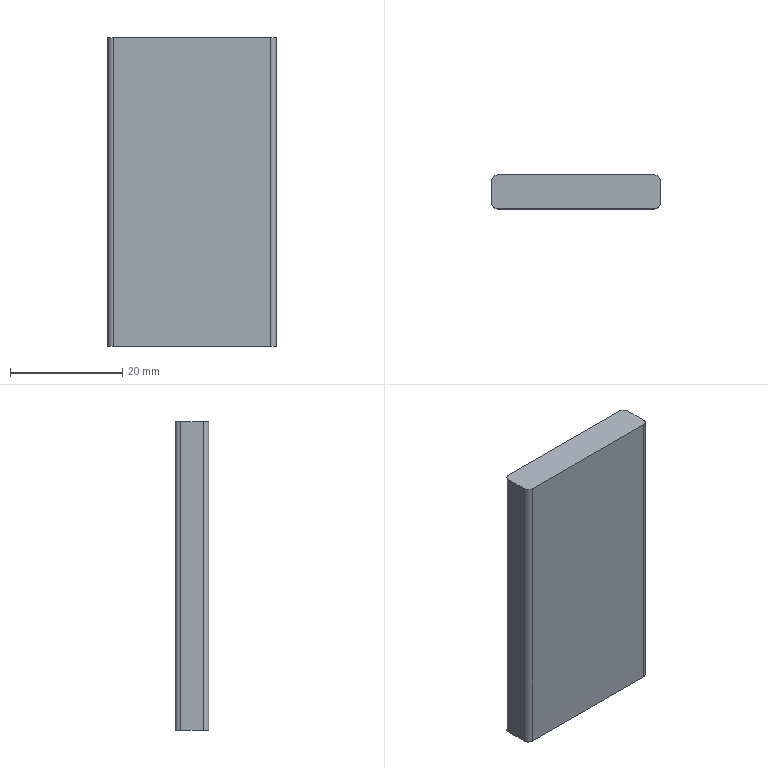Part | STEP file | 1 solid | 10 faces | box 29.97 x 5.97 x 55 mm | volume 9793 mm3 | plane 6 | cylinder 4 | commonest cylinder face diameters 2 x4
STEP:
#1=CARTESIAN_POINT('',(0.,0.,0.));
#2=DIRECTION('',(0.,0.,1.));
#3=DIRECTION('',(1.,0.,0.));
#4=AXIS2_PLACEMENT_3D('',#1,#2,#3);
#5=CARTESIAN_POINT('',(1284.232,493.53,43.619));
#6=VERTEX_POINT('',#5);
#7=CARTESIAN_POINT('',(1256.262,493.53,43.619));
#8=VERTEX_POINT('',#7);
#9=CARTESIAN_POINT('',(1285.247,493.53,43.619));
#10=DIRECTION('',(-1.,0.,0.));
#11=VECTOR('',#10,1.);
#12=LINE('',#9,#11);
#13=CARTESIAN_POINT('',(20687.4,-3520.314,43.619));
#14=DIRECTION('',(0.,0.,1.));
#15=DIRECTION('',(1.,0.,0.));
#16=AXIS2_PLACEMENT_3D('',#13,#14,#15);
#17=PLANE('',#16);
#18=CARTESIAN_POINT('',(-19402.153,4013.844));
#19=DIRECTION('',(-1.,0.));
#20=VECTOR('',#19,1.);
#21=LINE('',#18,#20);
#22=(GEOMETRIC_REPRESENTATION_CONTEXT(2)PARAMETRIC_REPRESENTATION_CONTEXT()REPRESENTATION_CONTEXT('',''));
#23=DEFINITIONAL_REPRESENTATION('',(#21),#22);
#24=PCURVE('',#17,#23);
#25=CARTESIAN_POINT('',(1285.247,493.53,426.319));
#26=DIRECTION('',(0.,-1.,0.));
#27=DIRECTION('',(0.,0.,1.));
#28=AXIS2_PLACEMENT_3D('',#25,#26,#27);
#29=PLANE('',#28);
#30=CARTESIAN_POINT('',(-382.7,0.));
#31=DIRECTION('',(0.,1.));
#32=VECTOR('',#31,1.);
#33=LINE('',#30,#32);
#34=(GEOMETRIC_REPRESENTATION_CONTEXT(2)PARAMETRIC_REPRESENTATION_CONTEXT()REPRESENTATION_CONTEXT('',''));
#35=DEFINITIONAL_REPRESENTATION('',(#33),#34);
#36=PCURVE('',#29,#35);
#37=SURFACE_CURVE('',#12,(#24,#36),.PCURVE_S1.);
#38=EDGE_CURVE('',#6,#8,#37,.T.);
#39=ORIENTED_EDGE('',*,*,#38,.T.);
#40=CARTESIAN_POINT('',(1255.262,492.53,43.619));
#41=VERTEX_POINT('',#40);
#42=CARTESIAN_POINT('',(1256.262,492.53,43.619));
#43=DIRECTION('',(0.,0.,1.));
#44=DIRECTION('',(-1.,0.,0.));
#45=AXIS2_PLACEMENT_3D('',#42,#43,#44);
#46=CIRCLE('',#45,1.);
#47=CARTESIAN_POINT('',(-19431.138,4012.844));
#48=DIRECTION('',(-1.,0.));
#49=AXIS2_PLACEMENT_2D('',#47,#48);
#50=CIRCLE('',#49,1.);
#51=(GEOMETRIC_REPRESENTATION_CONTEXT(2)PARAMETRIC_REPRESENTATION_CONTEXT()REPRESENTATION_CONTEXT('',''));
#52=DEFINITIONAL_REPRESENTATION('',(#50),#51);
#53=PCURVE('',#17,#52);
#54=CARTESIAN_POINT('',(1256.262,492.53,426.319));
#55=DIRECTION('',(0.,0.,-1.));
#56=DIRECTION('',(-1.,0.,0.));
#57=AXIS2_PLACEMENT_3D('',#54,#55,#56);
#58=CYLINDRICAL_SURFACE('',#57,1.);
#59=CARTESIAN_POINT('',(6.283,382.7));
#60=DIRECTION('',(-1.,0.));
#61=VECTOR('',#60,1.);
#62=LINE('',#59,#61);
#63=(GEOMETRIC_REPRESENTATION_CONTEXT(2)PARAMETRIC_REPRESENTATION_CONTEXT()REPRESENTATION_CONTEXT('',''));
#64=DEFINITIONAL_REPRESENTATION('',(#62),#63);
#65=PCURVE('',#58,#64);
#66=SURFACE_CURVE('',#46,(#53,#65),.PCURVE_S1.);
#67=EDGE_CURVE('',#8,#41,#66,.T.);
#68=ORIENTED_EDGE('',*,*,#67,.T.);
#69=CARTESIAN_POINT('',(1255.262,488.56,43.619));
#70=VERTEX_POINT('',#69);
#71=CARTESIAN_POINT('',(1255.262,493.545,43.619));
#72=DIRECTION('',(0.,-1.,0.));
#73=VECTOR('',#72,1.);
#74=LINE('',#71,#73);
#75=CARTESIAN_POINT('',(-19432.138,4013.859));
#76=DIRECTION('',(0.,-1.));
#77=VECTOR('',#76,1.);
#78=LINE('',#75,#77);
#79=(GEOMETRIC_REPRESENTATION_CONTEXT(2)PARAMETRIC_REPRESENTATION_CONTEXT()REPRESENTATION_CONTEXT('',''));
#80=DEFINITIONAL_REPRESENTATION('',(#78),#79);
#81=PCURVE('',#17,#80);
#82=CARTESIAN_POINT('',(1255.262,493.545,426.319));
#83=DIRECTION('',(1.,0.,0.));
#84=DIRECTION('',(0.,0.,-1.));
#85=AXIS2_PLACEMENT_3D('',#82,#83,#84);
#86=PLANE('',#85);
#87=CARTESIAN_POINT('',(382.7,0.));
#88=DIRECTION('',(0.,-1.));
#89=VECTOR('',#88,1.);
#90=LINE('',#87,#89);
#91=(GEOMETRIC_REPRESENTATION_CONTEXT(2)PARAMETRIC_REPRESENTATION_CONTEXT()REPRESENTATION_CONTEXT('',''));
#92=DEFINITIONAL_REPRESENTATION('',(#90),#91);
#93=PCURVE('',#86,#92);
#94=SURFACE_CURVE('',#74,(#81,#93),.PCURVE_S1.);
#95=EDGE_CURVE('',#41,#70,#94,.T.);
#96=ORIENTED_EDGE('',*,*,#95,.T.);
#97=CARTESIAN_POINT('',(1256.262,487.56,43.619));
#98=VERTEX_POINT('',#97);
#99=CARTESIAN_POINT('',(1256.262,488.56,43.619));
#100=DIRECTION('',(0.,0.,1.));
#101=DIRECTION('',(-1.,0.,0.));
#102=AXIS2_PLACEMENT_3D('',#99,#100,#101);
#103=CIRCLE('',#102,1.);
#104=CARTESIAN_POINT('',(-19431.138,4008.874));
#105=DIRECTION('',(-1.,0.));
#106=AXIS2_PLACEMENT_2D('',#104,#105);
#107=CIRCLE('',#106,1.);
#108=(GEOMETRIC_REPRESENTATION_CONTEXT(2)PARAMETRIC_REPRESENTATION_CONTEXT()REPRESENTATION_CONTEXT('',''));
#109=DEFINITIONAL_REPRESENTATION('',(#107),#108);
#110=PCURVE('',#17,#109);
#111=CARTESIAN_POINT('',(1256.262,488.56,426.319));
#112=DIRECTION('',(0.,0.,-1.));
#113=DIRECTION('',(-1.,0.,0.));
#114=AXIS2_PLACEMENT_3D('',#111,#112,#113);
#115=CYLINDRICAL_SURFACE('',#114,1.);
#116=CARTESIAN_POINT('',(6.283,382.7));
#117=DIRECTION('',(-1.,0.));
#118=VECTOR('',#117,1.);
#119=LINE('',#116,#118);
#120=(GEOMETRIC_REPRESENTATION_CONTEXT(2)PARAMETRIC_REPRESENTATION_CONTEXT()REPRESENTATION_CONTEXT('',''));
#121=DEFINITIONAL_REPRESENTATION('',(#119),#120);
#122=PCURVE('',#115,#121);
#123=SURFACE_CURVE('',#103,(#110,#122),.PCURVE_S1.);
#124=EDGE_CURVE('',#70,#98,#123,.T.);
#125=ORIENTED_EDGE('',*,*,#124,.T.);
#126=CARTESIAN_POINT('',(1284.232,487.56,43.619));
#127=VERTEX_POINT('',#126);
#128=CARTESIAN_POINT('',(1255.247,487.56,43.619));
#129=DIRECTION('',(1.,0.,0.));
#130=VECTOR('',#129,1.);
#131=LINE('',#128,#130);
#132=CARTESIAN_POINT('',(-19432.153,4007.874));
#133=DIRECTION('',(1.,0.));
#134=VECTOR('',#133,1.);
#135=LINE('',#132,#134);
#136=(GEOMETRIC_REPRESENTATION_CONTEXT(2)PARAMETRIC_REPRESENTATION_CONTEXT()REPRESENTATION_CONTEXT('',''));
#137=DEFINITIONAL_REPRESENTATION('',(#135),#136);
#138=PCURVE('',#17,#137);
#139=CARTESIAN_POINT('',(1255.247,487.56,426.319));
#140=DIRECTION('',(0.,1.,0.));
#141=DIRECTION('',(0.,0.,-1.));
#142=AXIS2_PLACEMENT_3D('',#139,#140,#141);
#143=PLANE('',#142);
#144=CARTESIAN_POINT('',(382.7,0.));
#145=DIRECTION('',(0.,-1.));
#146=VECTOR('',#145,1.);
#147=LINE('',#144,#146);
#148=(GEOMETRIC_REPRESENTATION_CONTEXT(2)PARAMETRIC_REPRESENTATION_CONTEXT()REPRESENTATION_CONTEXT('',''));
#149=DEFINITIONAL_REPRESENTATION('',(#147),#148);
#150=PCURVE('',#143,#149);
#151=SURFACE_CURVE('',#131,(#138,#150),.PCURVE_S1.);
#152=EDGE_CURVE('',#98,#127,#151,.T.);
#153=ORIENTED_EDGE('',*,*,#152,.T.);
#154=CARTESIAN_POINT('',(1285.232,488.56,43.619));
#155=VERTEX_POINT('',#154);
#156=CARTESIAN_POINT('',(1284.232,488.56,43.619));
#157=DIRECTION('',(0.,0.,1.));
#158=DIRECTION('',(-1.,0.,0.));
#159=AXIS2_PLACEMENT_3D('',#156,#157,#158);
#160=CIRCLE('',#159,1.);
#161=CARTESIAN_POINT('',(-19403.168,4008.874));
#162=DIRECTION('',(-1.,0.));
#163=AXIS2_PLACEMENT_2D('',#161,#162);
#164=CIRCLE('',#163,1.);
#165=(GEOMETRIC_REPRESENTATION_CONTEXT(2)PARAMETRIC_REPRESENTATION_CONTEXT()REPRESENTATION_CONTEXT('',''));
#166=DEFINITIONAL_REPRESENTATION('',(#164),#165);
#167=PCURVE('',#17,#166);
#168=CARTESIAN_POINT('',(1284.232,488.56,426.319));
#169=DIRECTION('',(0.,0.,-1.));
#170=DIRECTION('',(-1.,0.,0.));
#171=AXIS2_PLACEMENT_3D('',#168,#169,#170);
#172=CYLINDRICAL_SURFACE('',#171,1.);
#173=CARTESIAN_POINT('',(6.283,382.7));
#174=DIRECTION('',(-1.,0.));
#175=VECTOR('',#174,1.);
#176=LINE('',#173,#175);
#177=(GEOMETRIC_REPRESENTATION_CONTEXT(2)PARAMETRIC_REPRESENTATION_CONTEXT()REPRESENTATION_CONTEXT('',''));
#178=DEFINITIONAL_REPRESENTATION('',(#176),#177);
#179=PCURVE('',#172,#178);
#180=SURFACE_CURVE('',#160,(#167,#179),.PCURVE_S1.);
#181=EDGE_CURVE('',#127,#155,#180,.T.);
#182=ORIENTED_EDGE('',*,*,#181,.T.);
#183=CARTESIAN_POINT('',(1285.232,492.53,43.619));
#184=VERTEX_POINT('',#183);
#185=CARTESIAN_POINT('',(1285.232,487.545,43.619));
#186=DIRECTION('',(0.,1.,0.));
#187=VECTOR('',#186,1.);
#188=LINE('',#185,#187);
#189=CARTESIAN_POINT('',(-19402.168,4007.859));
#190=DIRECTION('',(0.,1.));
#191=VECTOR('',#190,1.);
#192=LINE('',#189,#191);
#193=(GEOMETRIC_REPRESENTATION_CONTEXT(2)PARAMETRIC_REPRESENTATION_CONTEXT()REPRESENTATION_CONTEXT('',''));
#194=DEFINITIONAL_REPRESENTATION('',(#192),#193);
#195=PCURVE('',#17,#194);
#196=CARTESIAN_POINT('',(1285.232,487.545,426.319));
#197=DIRECTION('',(-1.,0.,0.));
#198=DIRECTION('',(0.,0.,1.));
#199=AXIS2_PLACEMENT_3D('',#196,#197,#198);
#200=PLANE('',#199);
#201=CARTESIAN_POINT('',(-382.7,0.));
#202=DIRECTION('',(0.,1.));
#203=VECTOR('',#202,1.);
#204=LINE('',#201,#203);
#205=(GEOMETRIC_REPRESENTATION_CONTEXT(2)PARAMETRIC_REPRESENTATION_CONTEXT()REPRESENTATION_CONTEXT('',''));
#206=DEFINITIONAL_REPRESENTATION('',(#204),#205);
#207=PCURVE('',#200,#206);
#208=SURFACE_CURVE('',#188,(#195,#207),.PCURVE_S1.);
#209=EDGE_CURVE('',#155,#184,#208,.T.);
#210=ORIENTED_EDGE('',*,*,#209,.T.);
#211=CARTESIAN_POINT('',(1284.232,492.53,43.619));
#212=DIRECTION('',(0.,0.,1.));
#213=DIRECTION('',(-1.,0.,0.));
#214=AXIS2_PLACEMENT_3D('',#211,#212,#213);
#215=CIRCLE('',#214,1.);
#216=CARTESIAN_POINT('',(-19403.168,4012.844));
#217=DIRECTION('',(-1.,0.));
#218=AXIS2_PLACEMENT_2D('',#216,#217);
#219=CIRCLE('',#218,1.);
#220=(GEOMETRIC_REPRESENTATION_CONTEXT(2)PARAMETRIC_REPRESENTATION_CONTEXT()REPRESENTATION_CONTEXT('',''));
#221=DEFINITIONAL_REPRESENTATION('',(#219),#220);
#222=PCURVE('',#17,#221);
#223=CARTESIAN_POINT('',(1284.232,492.53,426.319));
#224=DIRECTION('',(0.,0.,-1.));
#225=DIRECTION('',(-1.,0.,0.));
#226=AXIS2_PLACEMENT_3D('',#223,#224,#225);
#227=CYLINDRICAL_SURFACE('',#226,1.);
#228=CARTESIAN_POINT('',(6.283,382.7));
#229=DIRECTION('',(-1.,0.));
#230=VECTOR('',#229,1.);
#231=LINE('',#228,#230);
#232=(GEOMETRIC_REPRESENTATION_CONTEXT(2)PARAMETRIC_REPRESENTATION_CONTEXT()REPRESENTATION_CONTEXT('',''));
#233=DEFINITIONAL_REPRESENTATION('',(#231),#232);
#234=PCURVE('',#227,#233);
#235=SURFACE_CURVE('',#215,(#222,#234),.PCURVE_S1.);
#236=EDGE_CURVE('',#184,#6,#235,.T.);
#237=ORIENTED_EDGE('',*,*,#236,.T.);
#238=EDGE_LOOP('',(#39,#68,#96,#125,#153,#182,#210,#237));
#239=FACE_BOUND('',#238,.T.);
#240=ADVANCED_FACE('',(#239),#17,.T.);
#241=CARTESIAN_POINT('',(1284.232,493.53,-11.381));
#242=VERTEX_POINT('',#241);
#243=CARTESIAN_POINT('',(1256.262,493.53,-11.381));
#244=VERTEX_POINT('',#243);
#245=CARTESIAN_POINT('',(1285.247,493.53,-11.381));
#246=DIRECTION('',(-1.,0.,0.));
#247=VECTOR('',#246,1.);
#248=LINE('',#245,#247);
#249=CARTESIAN_POINT('',(-437.7,0.));
#250=DIRECTION('',(0.,1.));
#251=VECTOR('',#250,1.);
#252=LINE('',#249,#251);
#253=(GEOMETRIC_REPRESENTATION_CONTEXT(2)PARAMETRIC_REPRESENTATION_CONTEXT()REPRESENTATION_CONTEXT('',''));
#254=DEFINITIONAL_REPRESENTATION('',(#252),#253);
#255=PCURVE('',#29,#254);
#256=CARTESIAN_POINT('',(18450.131,-3520.314,-11.381));
#257=DIRECTION('',(0.,0.,1.));
#258=DIRECTION('',(1.,0.,0.));
#259=AXIS2_PLACEMENT_3D('',#256,#257,#258);
#260=PLANE('',#259);
#261=CARTESIAN_POINT('',(-17164.884,4013.844));
#262=DIRECTION('',(-1.,0.));
#263=VECTOR('',#262,1.);
#264=LINE('',#261,#263);
#265=(GEOMETRIC_REPRESENTATION_CONTEXT(2)PARAMETRIC_REPRESENTATION_CONTEXT()REPRESENTATION_CONTEXT('',''));
#266=DEFINITIONAL_REPRESENTATION('',(#264),#265);
#267=PCURVE('',#260,#266);
#268=SURFACE_CURVE('',#248,(#255,#267),.PCURVE_S1.);
#269=EDGE_CURVE('',#242,#244,#268,.T.);
#270=ORIENTED_EDGE('',*,*,#269,.T.);
#271=CARTESIAN_POINT('',(1256.262,493.53,426.319));
#272=DIRECTION('',(0.,0.,1.));
#273=VECTOR('',#272,1.);
#274=LINE('',#271,#273);
#275=CARTESIAN_POINT('',(0.,28.985));
#276=DIRECTION('',(1.,0.));
#277=VECTOR('',#276,1.);
#278=LINE('',#275,#277);
#279=(GEOMETRIC_REPRESENTATION_CONTEXT(2)PARAMETRIC_REPRESENTATION_CONTEXT()REPRESENTATION_CONTEXT('',''));
#280=DEFINITIONAL_REPRESENTATION('',(#278),#279);
#281=PCURVE('',#29,#280);
#282=CARTESIAN_POINT('',(1.571,0.));
#283=DIRECTION('',(0.,-1.));
#284=VECTOR('',#283,1.);
#285=LINE('',#282,#284);
#286=(GEOMETRIC_REPRESENTATION_CONTEXT(2)PARAMETRIC_REPRESENTATION_CONTEXT()REPRESENTATION_CONTEXT('',''));
#287=DEFINITIONAL_REPRESENTATION('',(#285),#286);
#288=PCURVE('',#58,#287);
#289=SURFACE_CURVE('',#274,(#281,#288),.PCURVE_S1.);
#290=EDGE_CURVE('',#244,#8,#289,.T.);
#291=ORIENTED_EDGE('',*,*,#290,.T.);
#292=ORIENTED_EDGE('',*,*,#38,.F.);
#293=CARTESIAN_POINT('',(1284.232,493.53,426.319));
#294=DIRECTION('',(0.,0.,-1.));
#295=VECTOR('',#294,1.);
#296=LINE('',#293,#295);
#297=CARTESIAN_POINT('',(0.,1.015));
#298=DIRECTION('',(-1.,0.));
#299=VECTOR('',#298,1.);
#300=LINE('',#297,#299);
#301=(GEOMETRIC_REPRESENTATION_CONTEXT(2)PARAMETRIC_REPRESENTATION_CONTEXT()REPRESENTATION_CONTEXT('',''));
#302=DEFINITIONAL_REPRESENTATION('',(#300),#301);
#303=PCURVE('',#29,#302);
#304=CARTESIAN_POINT('',(1.571,0.));
#305=DIRECTION('',(0.,1.));
#306=VECTOR('',#305,1.);
#307=LINE('',#304,#306);
#308=(GEOMETRIC_REPRESENTATION_CONTEXT(2)PARAMETRIC_REPRESENTATION_CONTEXT()REPRESENTATION_CONTEXT('',''));
#309=DEFINITIONAL_REPRESENTATION('',(#307),#308);
#310=PCURVE('',#227,#309);
#311=SURFACE_CURVE('',#296,(#303,#310),.PCURVE_S1.);
#312=EDGE_CURVE('',#6,#242,#311,.T.);
#313=ORIENTED_EDGE('',*,*,#312,.T.);
#314=EDGE_LOOP('',(#270,#291,#292,#313));
#315=FACE_BOUND('',#314,.T.);
#316=ADVANCED_FACE('',(#315),#29,.F.);
#317=ORIENTED_EDGE('',*,*,#95,.F.);
#318=CARTESIAN_POINT('',(1255.262,492.53,-11.381));
#319=VERTEX_POINT('',#318);
#320=CARTESIAN_POINT('',(1255.262,492.53,426.319));
#321=DIRECTION('',(0.,0.,-1.));
#322=VECTOR('',#321,1.);
#323=LINE('',#320,#322);
#324=CARTESIAN_POINT('',(0.,-1.015));
#325=DIRECTION('',(1.,0.));
#326=VECTOR('',#325,1.);
#327=LINE('',#324,#326);
#328=(GEOMETRIC_REPRESENTATION_CONTEXT(2)PARAMETRIC_REPRESENTATION_CONTEXT()REPRESENTATION_CONTEXT('',''));
#329=DEFINITIONAL_REPRESENTATION('',(#327),#328);
#330=PCURVE('',#86,#329);
#331=CARTESIAN_POINT('',(0.,0.));
#332=DIRECTION('',(0.,1.));
#333=VECTOR('',#332,1.);
#334=LINE('',#331,#333);
#335=(GEOMETRIC_REPRESENTATION_CONTEXT(2)PARAMETRIC_REPRESENTATION_CONTEXT()REPRESENTATION_CONTEXT('',''));
#336=DEFINITIONAL_REPRESENTATION('',(#334),#335);
#337=PCURVE('',#58,#336);
#338=SURFACE_CURVE('',#323,(#330,#337),.PCURVE_S1.);
#339=EDGE_CURVE('',#41,#319,#338,.T.);
#340=ORIENTED_EDGE('',*,*,#339,.T.);
#341=CARTESIAN_POINT('',(1255.262,488.56,-11.381));
#342=VERTEX_POINT('',#341);
#343=CARTESIAN_POINT('',(1255.262,493.545,-11.381));
#344=DIRECTION('',(0.,-1.,0.));
#345=VECTOR('',#344,1.);
#346=LINE('',#343,#345);
#347=CARTESIAN_POINT('',(437.7,0.));
#348=DIRECTION('',(0.,-1.));
#349=VECTOR('',#348,1.);
#350=LINE('',#347,#349);
#351=(GEOMETRIC_REPRESENTATION_CONTEXT(2)PARAMETRIC_REPRESENTATION_CONTEXT()REPRESENTATION_CONTEXT('',''));
#352=DEFINITIONAL_REPRESENTATION('',(#350),#351);
#353=PCURVE('',#86,#352);
#354=CARTESIAN_POINT('',(-17194.869,4013.859));
#355=DIRECTION('',(0.,-1.));
#356=VECTOR('',#355,1.);
#357=LINE('',#354,#356);
#358=(GEOMETRIC_REPRESENTATION_CONTEXT(2)PARAMETRIC_REPRESENTATION_CONTEXT()REPRESENTATION_CONTEXT('',''));
#359=DEFINITIONAL_REPRESENTATION('',(#357),#358);
#360=PCURVE('',#260,#359);
#361=SURFACE_CURVE('',#346,(#353,#360),.PCURVE_S1.);
#362=EDGE_CURVE('',#319,#342,#361,.T.);
#363=ORIENTED_EDGE('',*,*,#362,.T.);
#364=CARTESIAN_POINT('',(1255.262,488.56,426.319));
#365=DIRECTION('',(0.,0.,1.));
#366=VECTOR('',#365,1.);
#367=LINE('',#364,#366);
#368=CARTESIAN_POINT('',(0.,-4.985));
#369=DIRECTION('',(-1.,0.));
#370=VECTOR('',#369,1.);
#371=LINE('',#368,#370);
#372=(GEOMETRIC_REPRESENTATION_CONTEXT(2)PARAMETRIC_REPRESENTATION_CONTEXT()REPRESENTATION_CONTEXT('',''));
#373=DEFINITIONAL_REPRESENTATION('',(#371),#372);
#374=PCURVE('',#86,#373);
#375=CARTESIAN_POINT('',(6.283,0.));
#376=DIRECTION('',(0.,-1.));
#377=VECTOR('',#376,1.);
#378=LINE('',#375,#377);
#379=(GEOMETRIC_REPRESENTATION_CONTEXT(2)PARAMETRIC_REPRESENTATION_CONTEXT()REPRESENTATION_CONTEXT('',''));
#380=DEFINITIONAL_REPRESENTATION('',(#378),#379);
#381=PCURVE('',#115,#380);
#382=SURFACE_CURVE('',#367,(#374,#381),.PCURVE_S1.);
#383=EDGE_CURVE('',#342,#70,#382,.T.);
#384=ORIENTED_EDGE('',*,*,#383,.T.);
#385=EDGE_LOOP('',(#317,#340,#363,#384));
#386=FACE_BOUND('',#385,.T.);
#387=ADVANCED_FACE('',(#386),#86,.F.);
#388=ORIENTED_EDGE('',*,*,#152,.F.);
#389=CARTESIAN_POINT('',(1256.262,487.56,-11.381));
#390=VERTEX_POINT('',#389);
#391=CARTESIAN_POINT('',(1256.262,487.56,426.319));
#392=DIRECTION('',(0.,0.,-1.));
#393=VECTOR('',#392,1.);
#394=LINE('',#391,#393);
#395=CARTESIAN_POINT('',(0.,-1.015));
#396=DIRECTION('',(1.,0.));
#397=VECTOR('',#396,1.);
#398=LINE('',#395,#397);
#399=(GEOMETRIC_REPRESENTATION_CONTEXT(2)PARAMETRIC_REPRESENTATION_CONTEXT()REPRESENTATION_CONTEXT('',''));
#400=DEFINITIONAL_REPRESENTATION('',(#398),#399);
#401=PCURVE('',#143,#400);
#402=CARTESIAN_POINT('',(4.712,0.));
#403=DIRECTION('',(0.,1.));
#404=VECTOR('',#403,1.);
#405=LINE('',#402,#404);
#406=(GEOMETRIC_REPRESENTATION_CONTEXT(2)PARAMETRIC_REPRESENTATION_CONTEXT()REPRESENTATION_CONTEXT('',''));
#407=DEFINITIONAL_REPRESENTATION('',(#405),#406);
#408=PCURVE('',#115,#407);
#409=SURFACE_CURVE('',#394,(#401,#408),.PCURVE_S1.);
#410=EDGE_CURVE('',#98,#390,#409,.T.);
#411=ORIENTED_EDGE('',*,*,#410,.T.);
#412=CARTESIAN_POINT('',(1284.232,487.56,-11.381));
#413=VERTEX_POINT('',#412);
#414=CARTESIAN_POINT('',(1255.247,487.56,-11.381));
#415=DIRECTION('',(1.,0.,0.));
#416=VECTOR('',#415,1.);
#417=LINE('',#414,#416);
#418=CARTESIAN_POINT('',(437.7,0.));
#419=DIRECTION('',(0.,-1.));
#420=VECTOR('',#419,1.);
#421=LINE('',#418,#420);
#422=(GEOMETRIC_REPRESENTATION_CONTEXT(2)PARAMETRIC_REPRESENTATION_CONTEXT()REPRESENTATION_CONTEXT('',''));
#423=DEFINITIONAL_REPRESENTATION('',(#421),#422);
#424=PCURVE('',#143,#423);
#425=CARTESIAN_POINT('',(-17194.884,4007.874));
#426=DIRECTION('',(1.,0.));
#427=VECTOR('',#426,1.);
#428=LINE('',#425,#427);
#429=(GEOMETRIC_REPRESENTATION_CONTEXT(2)PARAMETRIC_REPRESENTATION_CONTEXT()REPRESENTATION_CONTEXT('',''));
#430=DEFINITIONAL_REPRESENTATION('',(#428),#429);
#431=PCURVE('',#260,#430);
#432=SURFACE_CURVE('',#417,(#424,#431),.PCURVE_S1.);
#433=EDGE_CURVE('',#390,#413,#432,.T.);
#434=ORIENTED_EDGE('',*,*,#433,.T.);
#435=CARTESIAN_POINT('',(1284.232,487.56,426.319));
#436=DIRECTION('',(0.,0.,1.));
#437=VECTOR('',#436,1.);
#438=LINE('',#435,#437);
#439=CARTESIAN_POINT('',(0.,-28.985));
#440=DIRECTION('',(-1.,0.));
#441=VECTOR('',#440,1.);
#442=LINE('',#439,#441);
#443=(GEOMETRIC_REPRESENTATION_CONTEXT(2)PARAMETRIC_REPRESENTATION_CONTEXT()REPRESENTATION_CONTEXT('',''));
#444=DEFINITIONAL_REPRESENTATION('',(#442),#443);
#445=PCURVE('',#143,#444);
#446=CARTESIAN_POINT('',(4.712,0.));
#447=DIRECTION('',(0.,-1.));
#448=VECTOR('',#447,1.);
#449=LINE('',#446,#448);
#450=(GEOMETRIC_REPRESENTATION_CONTEXT(2)PARAMETRIC_REPRESENTATION_CONTEXT()REPRESENTATION_CONTEXT('',''));
#451=DEFINITIONAL_REPRESENTATION('',(#449),#450);
#452=PCURVE('',#172,#451);
#453=SURFACE_CURVE('',#438,(#445,#452),.PCURVE_S1.);
#454=EDGE_CURVE('',#413,#127,#453,.T.);
#455=ORIENTED_EDGE('',*,*,#454,.T.);
#456=EDGE_LOOP('',(#388,#411,#434,#455));
#457=FACE_BOUND('',#456,.T.);
#458=ADVANCED_FACE('',(#457),#143,.F.);
#459=CARTESIAN_POINT('',(1285.232,488.56,-11.381));
#460=VERTEX_POINT('',#459);
#461=CARTESIAN_POINT('',(1285.232,492.53,-11.381));
#462=VERTEX_POINT('',#461);
#463=CARTESIAN_POINT('',(1285.232,487.545,-11.381));
#464=DIRECTION('',(0.,1.,0.));
#465=VECTOR('',#464,1.);
#466=LINE('',#463,#465);
#467=CARTESIAN_POINT('',(-437.7,0.));
#468=DIRECTION('',(0.,1.));
#469=VECTOR('',#468,1.);
#470=LINE('',#467,#469);
#471=(GEOMETRIC_REPRESENTATION_CONTEXT(2)PARAMETRIC_REPRESENTATION_CONTEXT()REPRESENTATION_CONTEXT('',''));
#472=DEFINITIONAL_REPRESENTATION('',(#470),#471);
#473=PCURVE('',#200,#472);
#474=CARTESIAN_POINT('',(-17164.899,4007.859));
#475=DIRECTION('',(0.,1.));
#476=VECTOR('',#475,1.);
#477=LINE('',#474,#476);
#478=(GEOMETRIC_REPRESENTATION_CONTEXT(2)PARAMETRIC_REPRESENTATION_CONTEXT()REPRESENTATION_CONTEXT('',''));
#479=DEFINITIONAL_REPRESENTATION('',(#477),#478);
#480=PCURVE('',#260,#479);
#481=SURFACE_CURVE('',#466,(#473,#480),.PCURVE_S1.);
#482=EDGE_CURVE('',#460,#462,#481,.T.);
#483=ORIENTED_EDGE('',*,*,#482,.T.);
#484=CARTESIAN_POINT('',(1285.232,492.53,426.319));
#485=DIRECTION('',(0.,0.,1.));
#486=VECTOR('',#485,1.);
#487=LINE('',#484,#486);
#488=CARTESIAN_POINT('',(0.,4.985));
#489=DIRECTION('',(1.,0.));
#490=VECTOR('',#489,1.);
#491=LINE('',#488,#490);
#492=(GEOMETRIC_REPRESENTATION_CONTEXT(2)PARAMETRIC_REPRESENTATION_CONTEXT()REPRESENTATION_CONTEXT('',''));
#493=DEFINITIONAL_REPRESENTATION('',(#491),#492);
#494=PCURVE('',#200,#493);
#495=CARTESIAN_POINT('',(3.142,0.));
#496=DIRECTION('',(0.,-1.));
#497=VECTOR('',#496,1.);
#498=LINE('',#495,#497);
#499=(GEOMETRIC_REPRESENTATION_CONTEXT(2)PARAMETRIC_REPRESENTATION_CONTEXT()REPRESENTATION_CONTEXT('',''));
#500=DEFINITIONAL_REPRESENTATION('',(#498),#499);
#501=PCURVE('',#227,#500);
#502=SURFACE_CURVE('',#487,(#494,#501),.PCURVE_S1.);
#503=EDGE_CURVE('',#462,#184,#502,.T.);
#504=ORIENTED_EDGE('',*,*,#503,.T.);
#505=ORIENTED_EDGE('',*,*,#209,.F.);
#506=CARTESIAN_POINT('',(1285.232,488.56,426.319));
#507=DIRECTION('',(0.,0.,-1.));
#508=VECTOR('',#507,1.);
#509=LINE('',#506,#508);
#510=CARTESIAN_POINT('',(0.,1.015));
#511=DIRECTION('',(-1.,0.));
#512=VECTOR('',#511,1.);
#513=LINE('',#510,#512);
#514=(GEOMETRIC_REPRESENTATION_CONTEXT(2)PARAMETRIC_REPRESENTATION_CONTEXT()REPRESENTATION_CONTEXT('',''));
#515=DEFINITIONAL_REPRESENTATION('',(#513),#514);
#516=PCURVE('',#200,#515);
#517=CARTESIAN_POINT('',(3.142,0.));
#518=DIRECTION('',(0.,1.));
#519=VECTOR('',#518,1.);
#520=LINE('',#517,#519);
#521=(GEOMETRIC_REPRESENTATION_CONTEXT(2)PARAMETRIC_REPRESENTATION_CONTEXT()REPRESENTATION_CONTEXT('',''));
#522=DEFINITIONAL_REPRESENTATION('',(#520),#521);
#523=PCURVE('',#172,#522);
#524=SURFACE_CURVE('',#509,(#516,#523),.PCURVE_S1.);
#525=EDGE_CURVE('',#155,#460,#524,.T.);
#526=ORIENTED_EDGE('',*,*,#525,.T.);
#527=EDGE_LOOP('',(#483,#504,#505,#526));
#528=FACE_BOUND('',#527,.T.);
#529=ADVANCED_FACE('',(#528),#200,.F.);
#530=ORIENTED_EDGE('',*,*,#362,.F.);
#531=CARTESIAN_POINT('',(1256.262,492.53,-11.381));
#532=DIRECTION('',(0.,0.,-1.));
#533=DIRECTION('',(1.,0.,0.));
#534=AXIS2_PLACEMENT_3D('',#531,#532,#533);
#535=CIRCLE('',#534,1.);
#536=CARTESIAN_POINT('',(-17192.869,4012.844));
#537=CARTESIAN_POINT('',(-17192.869,4011.112));
#538=CARTESIAN_POINT('',(-17194.369,4011.978));
#539=CARTESIAN_POINT('',(-17195.869,4012.844));
#540=CARTESIAN_POINT('',(-17194.369,4013.71));
#541=CARTESIAN_POINT('',(-17192.869,4014.576));
#542=CARTESIAN_POINT('',(-17192.869,4012.844));
#543=(BOUNDED_CURVE()B_SPLINE_CURVE(2,(#536,#537,#538,#539,#540,#541,#542),.UNSPECIFIED.,.T.,.F.)B_SPLINE_CURVE_WITH_KNOTS((1,2,2,2,2,1),(-2.094,0.,2.094,4.189,6.283,8.378),.UNSPECIFIED.)CURVE()GEOMETRIC_REPRESENTATION_ITEM()RATIONAL_B_SPLINE_CURVE((1.,0.5,1.,0.5,1.,0.5,1.))REPRESENTATION_ITEM(''));
#544=(GEOMETRIC_REPRESENTATION_CONTEXT(2)PARAMETRIC_REPRESENTATION_CONTEXT()REPRESENTATION_CONTEXT('',''));
#545=DEFINITIONAL_REPRESENTATION('',(#543),#544);
#546=PCURVE('',#260,#545);
#547=CARTESIAN_POINT('',(-3.142,437.7));
#548=DIRECTION('',(1.,0.));
#549=VECTOR('',#548,1.);
#550=LINE('',#547,#549);
#551=(GEOMETRIC_REPRESENTATION_CONTEXT(2)PARAMETRIC_REPRESENTATION_CONTEXT()REPRESENTATION_CONTEXT('',''));
#552=DEFINITIONAL_REPRESENTATION('',(#550),#551);
#553=PCURVE('',#58,#552);
#554=SURFACE_CURVE('',#535,(#546,#553),.PCURVE_S1.);
#555=EDGE_CURVE('',#319,#244,#554,.T.);
#556=ORIENTED_EDGE('',*,*,#555,.T.);
#557=ORIENTED_EDGE('',*,*,#269,.F.);
#558=CARTESIAN_POINT('',(1284.232,492.53,-11.381));
#559=DIRECTION('',(0.,0.,-1.));
#560=DIRECTION('',(1.,0.,0.));
#561=AXIS2_PLACEMENT_3D('',#558,#559,#560);
#562=CIRCLE('',#561,1.);
#563=CARTESIAN_POINT('',(-17164.899,4012.844));
#564=CARTESIAN_POINT('',(-17164.899,4011.112));
#565=CARTESIAN_POINT('',(-17166.399,4011.978));
#566=CARTESIAN_POINT('',(-17167.899,4012.844));
#567=CARTESIAN_POINT('',(-17166.399,4013.71));
#568=CARTESIAN_POINT('',(-17164.899,4014.576));
#569=CARTESIAN_POINT('',(-17164.899,4012.844));
#570=(BOUNDED_CURVE()B_SPLINE_CURVE(2,(#563,#564,#565,#566,#567,#568,#569),.UNSPECIFIED.,.T.,.F.)B_SPLINE_CURVE_WITH_KNOTS((1,2,2,2,2,1),(-2.094,0.,2.094,4.189,6.283,8.378),.UNSPECIFIED.)CURVE()GEOMETRIC_REPRESENTATION_ITEM()RATIONAL_B_SPLINE_CURVE((1.,0.5,1.,0.5,1.,0.5,1.))REPRESENTATION_ITEM(''));
#571=(GEOMETRIC_REPRESENTATION_CONTEXT(2)PARAMETRIC_REPRESENTATION_CONTEXT()REPRESENTATION_CONTEXT('',''));
#572=DEFINITIONAL_REPRESENTATION('',(#570),#571);
#573=PCURVE('',#260,#572);
#574=CARTESIAN_POINT('',(-3.142,437.7));
#575=DIRECTION('',(1.,0.));
#576=VECTOR('',#575,1.);
#577=LINE('',#574,#576);
#578=(GEOMETRIC_REPRESENTATION_CONTEXT(2)PARAMETRIC_REPRESENTATION_CONTEXT()REPRESENTATION_CONTEXT('',''));
#579=DEFINITIONAL_REPRESENTATION('',(#577),#578);
#580=PCURVE('',#227,#579);
#581=SURFACE_CURVE('',#562,(#573,#580),.PCURVE_S1.);
#582=EDGE_CURVE('',#242,#462,#581,.T.);
#583=ORIENTED_EDGE('',*,*,#582,.T.);
#584=ORIENTED_EDGE('',*,*,#482,.F.);
#585=CARTESIAN_POINT('',(1284.232,488.56,-11.381));
#586=DIRECTION('',(0.,0.,-1.));
#587=DIRECTION('',(1.,0.,0.));
#588=AXIS2_PLACEMENT_3D('',#585,#586,#587);
#589=CIRCLE('',#588,1.);
#590=CARTESIAN_POINT('',(-17164.899,4008.874));
#591=CARTESIAN_POINT('',(-17164.899,4007.142));
#592=CARTESIAN_POINT('',(-17166.399,4008.008));
#593=CARTESIAN_POINT('',(-17167.899,4008.874));
#594=CARTESIAN_POINT('',(-17166.399,4009.74));
#595=CARTESIAN_POINT('',(-17164.899,4010.606));
#596=CARTESIAN_POINT('',(-17164.899,4008.874));
#597=(BOUNDED_CURVE()B_SPLINE_CURVE(2,(#590,#591,#592,#593,#594,#595,#596),.UNSPECIFIED.,.T.,.F.)B_SPLINE_CURVE_WITH_KNOTS((1,2,2,2,2,1),(-2.094,0.,2.094,4.189,6.283,8.378),.UNSPECIFIED.)CURVE()GEOMETRIC_REPRESENTATION_ITEM()RATIONAL_B_SPLINE_CURVE((1.,0.5,1.,0.5,1.,0.5,1.))REPRESENTATION_ITEM(''));
#598=(GEOMETRIC_REPRESENTATION_CONTEXT(2)PARAMETRIC_REPRESENTATION_CONTEXT()REPRESENTATION_CONTEXT('',''));
#599=DEFINITIONAL_REPRESENTATION('',(#597),#598);
#600=PCURVE('',#260,#599);
#601=CARTESIAN_POINT('',(3.142,437.7));
#602=DIRECTION('',(1.,0.));
#603=VECTOR('',#602,1.);
#604=LINE('',#601,#603);
#605=(GEOMETRIC_REPRESENTATION_CONTEXT(2)PARAMETRIC_REPRESENTATION_CONTEXT()REPRESENTATION_CONTEXT('',''));
#606=DEFINITIONAL_REPRESENTATION('',(#604),#605);
#607=PCURVE('',#172,#606);
#608=SURFACE_CURVE('',#589,(#600,#607),.PCURVE_S1.);
#609=EDGE_CURVE('',#460,#413,#608,.T.);
#610=ORIENTED_EDGE('',*,*,#609,.T.);
#611=ORIENTED_EDGE('',*,*,#433,.F.);
#612=CARTESIAN_POINT('',(1256.262,488.56,-11.381));
#613=DIRECTION('',(0.,0.,-1.));
#614=DIRECTION('',(1.,0.,0.));
#615=AXIS2_PLACEMENT_3D('',#612,#613,#614);
#616=CIRCLE('',#615,1.);
#617=CARTESIAN_POINT('',(-17192.869,4008.874));
#618=CARTESIAN_POINT('',(-17192.869,4007.142));
#619=CARTESIAN_POINT('',(-17194.369,4008.008));
#620=CARTESIAN_POINT('',(-17195.869,4008.874));
#621=CARTESIAN_POINT('',(-17194.369,4009.74));
#622=CARTESIAN_POINT('',(-17192.869,4010.606));
#623=CARTESIAN_POINT('',(-17192.869,4008.874));
#624=(BOUNDED_CURVE()B_SPLINE_CURVE(2,(#617,#618,#619,#620,#621,#622,#623),.UNSPECIFIED.,.T.,.F.)B_SPLINE_CURVE_WITH_KNOTS((1,2,2,2,2,1),(-2.094,0.,2.094,4.189,6.283,8.378),.UNSPECIFIED.)CURVE()GEOMETRIC_REPRESENTATION_ITEM()RATIONAL_B_SPLINE_CURVE((1.,0.5,1.,0.5,1.,0.5,1.))REPRESENTATION_ITEM(''));
#625=(GEOMETRIC_REPRESENTATION_CONTEXT(2)PARAMETRIC_REPRESENTATION_CONTEXT()REPRESENTATION_CONTEXT('',''));
#626=DEFINITIONAL_REPRESENTATION('',(#624),#625);
#627=PCURVE('',#260,#626);
#628=CARTESIAN_POINT('',(3.142,437.7));
#629=DIRECTION('',(1.,0.));
#630=VECTOR('',#629,1.);
#631=LINE('',#628,#630);
#632=(GEOMETRIC_REPRESENTATION_CONTEXT(2)PARAMETRIC_REPRESENTATION_CONTEXT()REPRESENTATION_CONTEXT('',''));
#633=DEFINITIONAL_REPRESENTATION('',(#631),#632);
#634=PCURVE('',#115,#633);
#635=SURFACE_CURVE('',#616,(#627,#634),.PCURVE_S1.);
#636=EDGE_CURVE('',#390,#342,#635,.T.);
#637=ORIENTED_EDGE('',*,*,#636,.T.);
#638=EDGE_LOOP('',(#530,#556,#557,#583,#584,#610,#611,#637));
#639=FACE_BOUND('',#638,.T.);
#640=ADVANCED_FACE('',(#639),#260,.F.);
#641=ORIENTED_EDGE('',*,*,#67,.F.);
#642=ORIENTED_EDGE('',*,*,#290,.F.);
#643=ORIENTED_EDGE('',*,*,#555,.F.);
#644=ORIENTED_EDGE('',*,*,#339,.F.);
#645=EDGE_LOOP('',(#641,#642,#643,#644));
#646=FACE_BOUND('',#645,.T.);
#647=ADVANCED_FACE('',(#646),#58,.T.);
#648=ORIENTED_EDGE('',*,*,#124,.F.);
#649=ORIENTED_EDGE('',*,*,#383,.F.);
#650=ORIENTED_EDGE('',*,*,#636,.F.);
#651=ORIENTED_EDGE('',*,*,#410,.F.);
#652=EDGE_LOOP('',(#648,#649,#650,#651));
#653=FACE_BOUND('',#652,.T.);
#654=ADVANCED_FACE('',(#653),#115,.T.);
#655=ORIENTED_EDGE('',*,*,#236,.F.);
#656=ORIENTED_EDGE('',*,*,#503,.F.);
#657=ORIENTED_EDGE('',*,*,#582,.F.);
#658=ORIENTED_EDGE('',*,*,#312,.F.);
#659=EDGE_LOOP('',(#655,#656,#657,#658));
#660=FACE_BOUND('',#659,.T.);
#661=ADVANCED_FACE('',(#660),#227,.T.);
#662=ORIENTED_EDGE('',*,*,#181,.F.);
#663=ORIENTED_EDGE('',*,*,#454,.F.);
#664=ORIENTED_EDGE('',*,*,#609,.F.);
#665=ORIENTED_EDGE('',*,*,#525,.F.);
#666=EDGE_LOOP('',(#662,#663,#664,#665));
#667=FACE_BOUND('',#666,.T.);
#668=ADVANCED_FACE('',(#667),#172,.T.);
#669=CLOSED_SHELL('',(#240,#316,#387,#458,#529,#640,#647,#654,#661,#668));
#670=MANIFOLD_SOLID_BREP('',#669);
#671=(LENGTH_UNIT()NAMED_UNIT(*)SI_UNIT(.MILLI.,.METRE.));
#672=UNCERTAINTY_MEASURE_WITH_UNIT(LENGTH_MEASURE(0.0000001),#671,'','');
#673=(NAMED_UNIT(*)PLANE_ANGLE_UNIT()SI_UNIT($,.RADIAN.));
#674=(NAMED_UNIT(*)SI_UNIT($,.STERADIAN.)SOLID_ANGLE_UNIT());
#675=(GEOMETRIC_REPRESENTATION_CONTEXT(3)GLOBAL_UNCERTAINTY_ASSIGNED_CONTEXT((#672))GLOBAL_UNIT_ASSIGNED_CONTEXT((#671,#673,#674))REPRESENTATION_CONTEXT('',''));
#676=ADVANCED_BREP_SHAPE_REPRESENTATION('',(#4,#670),#675);